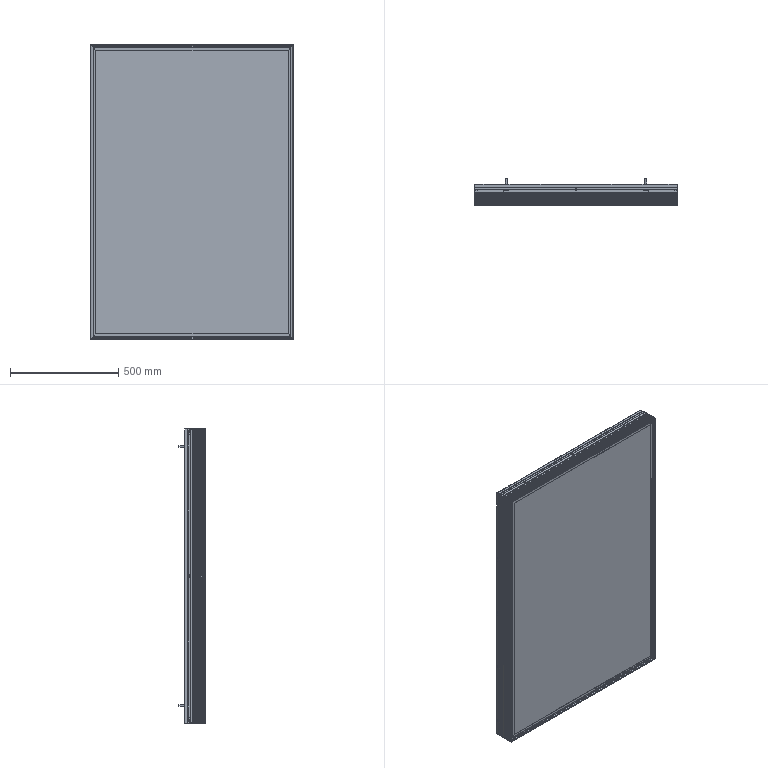Part | SolidWorks | 71 solids | 4172 faces | volume 153624719 mm3 | plane 2369 | cylinder 1643 | spline 104 | cone 56 | commonest cylinder face diameters 4.2 x581 7 x330 0.4 x198 2.4 x140 11 x118 20 x52